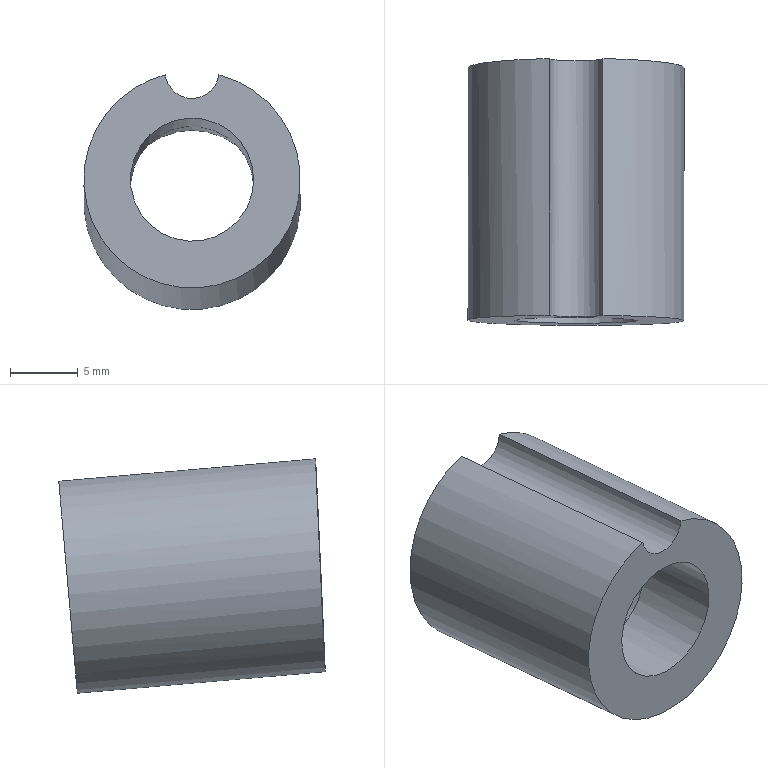Part | NX | features EKSD 16-20-9.100 2 | 1 solid | 7 faces | box 16 x 19.691 x 17.35 mm | volume 2155 mm3 | cylinder 4 | plane 3 | commonest cylinder face diameters 4 x1 9.1 x1 10.6 x1 16 x1
STEP:
#1=CARTESIAN_POINT('',(196.742,-27.508,-41.113));
#2=VERTEX_POINT('',#1);
#3=CARTESIAN_POINT('',(200.711,-27.508,-41.113));
#4=VERTEX_POINT('',#3);
#5=CARTESIAN_POINT('',(198.727,-27.486,-40.864));
#6=DIRECTION('',(0.,-0.9962,0.08716));
#7=DIRECTION('',(0.,-0.08716,-0.9962));
#8=AXIS2_PLACEMENT_3D('',#5,#6,#7);
#9=CIRCLE('',#8,2.);
#10=EDGE_CURVE('',#2,#4,#9,.T.);
#11=ORIENTED_EDGE('',*,*,#10,.T.);
#12=CARTESIAN_POINT('',(198.727,-28.184,-48.834));
#13=DIRECTION('',(0.,-0.9962,0.08716));
#14=DIRECTION('',(0.,-0.08716,-0.9962));
#15=AXIS2_PLACEMENT_3D('',#12,#13,#14);
#16=CIRCLE('',#15,8.);
#17=EDGE_CURVE('',#2,#4,#16,.T.);
#18=ORIENTED_EDGE('',*,*,#17,.F.);
#19=EDGE_LOOP('',(#11,#18));
#20=FACE_BOUND('',#19,.T.);
#21=CARTESIAN_POINT('',(198.727,-27.722,-43.554));
#22=VERTEX_POINT('',#21);
#23=CARTESIAN_POINT('',(198.727,-28.184,-48.834));
#24=DIRECTION('',(0.,0.9962,-0.08716));
#25=DIRECTION('',(0.,0.08716,0.9962));
#26=AXIS2_PLACEMENT_3D('',#23,#24,#25);
#27=CIRCLE('',#26,5.3);
#28=EDGE_CURVE('',#22,#22,#27,.T.);
#29=ORIENTED_EDGE('',*,*,#28,.F.);
#30=EDGE_LOOP('',(#29));
#31=FACE_BOUND('',#30,.T.);
#32=CARTESIAN_POINT('',(198.727,-28.184,-48.834));
#33=DIRECTION('',(0.,0.9962,-0.08716));
#34=DIRECTION('',(0.,0.08716,0.9962));
#35=AXIS2_PLACEMENT_3D('',#32,#33,#34);
#36=PLANE('',#35);
#37=ADVANCED_FACE('',(#20,#31),#36,.T.);
#38=CARTESIAN_POINT('',(200.711,-46.486,-39.453));
#39=VERTEX_POINT('',#38);
#40=CARTESIAN_POINT('',(196.742,-46.478,-39.454));
#41=VERTEX_POINT('',#40);
#42=CARTESIAN_POINT('',(198.727,-46.471,-39.203));
#43=DIRECTION('',(0.001957,0.999,-0.04546));
#44=DIRECTION('',(-0.04675,-0.04532,-0.9979));
#45=AXIS2_PLACEMENT_3D('',#42,#43,#44);
#46=ELLIPSE('',#45,2.002,2.);
#47=EDGE_CURVE('',#39,#41,#46,.T.);
#48=ORIENTED_EDGE('',*,*,#47,.T.);
#49=CARTESIAN_POINT('',(198.727,-46.835,-47.202));
#50=DIRECTION('',(0.001957,0.999,-0.04546));
#51=DIRECTION('',(-0.04675,-0.04532,-0.9979));
#52=AXIS2_PLACEMENT_3D('',#49,#50,#51);
#53=ELLIPSE('',#52,8.007,8.);
#54=EDGE_CURVE('',#39,#41,#53,.T.);
#55=ORIENTED_EDGE('',*,*,#54,.F.);
#56=EDGE_LOOP('',(#48,#55));
#57=FACE_BOUND('',#56,.T.);
#58=CARTESIAN_POINT('',(198.514,-47.041,-51.746));
#59=VERTEX_POINT('',#58);
#60=CARTESIAN_POINT('',(198.727,-46.835,-47.202));
#61=DIRECTION('',(0.001957,0.999,-0.04546));
#62=DIRECTION('',(-0.04675,-0.04532,-0.9979));
#63=AXIS2_PLACEMENT_3D('',#60,#61,#62);
#64=ELLIPSE('',#63,4.554,4.55);
#65=EDGE_CURVE('',#59,#59,#64,.F.);
#66=ORIENTED_EDGE('',*,*,#65,.F.);
#67=EDGE_LOOP('',(#66));
#68=FACE_BOUND('',#67,.T.);
#69=CARTESIAN_POINT('',(128.811,-48.589,-88.763));
#70=DIRECTION('',(0.001957,0.999,-0.04546));
#71=DIRECTION('',(0.06617,0.04523,0.9968));
#72=AXIS2_PLACEMENT_3D('',#69,#70,#71);
#73=PLANE('',#72);
#74=ADVANCED_FACE('',(#57,#68),#73,.F.);
#75=CARTESIAN_POINT('',(200.711,-37.47,-40.242));
#76=DIRECTION('',(0.,0.9962,-0.08716));
#77=VECTOR('',#76,1000.);
#78=LINE('',#75,#77);
#79=EDGE_CURVE('',#39,#4,#78,.T.);
#80=ORIENTED_EDGE('',*,*,#79,.F.);
#81=ORIENTED_EDGE('',*,*,#54,.T.);
#82=CARTESIAN_POINT('',(196.742,-37.47,-40.242));
#83=DIRECTION('',(0.,0.9962,-0.08716));
#84=VECTOR('',#83,1000.);
#85=LINE('',#82,#84);
#86=EDGE_CURVE('',#2,#41,#85,.F.);
#87=ORIENTED_EDGE('',*,*,#86,.F.);
#88=ORIENTED_EDGE('',*,*,#17,.T.);
#89=EDGE_LOOP('',(#80,#81,#87,#88));
#90=FACE_BOUND('',#89,.T.);
#91=CARTESIAN_POINT('',(198.727,-48.107,-47.091));
#92=DIRECTION('',(0.,0.9962,-0.08716));
#93=DIRECTION('',(0.,0.08716,0.9962));
#94=AXIS2_PLACEMENT_3D('',#91,#92,#93);
#95=CYLINDRICAL_SURFACE('',#94,8.);
#96=ADVANCED_FACE('',(#90),#95,.T.);
#97=CARTESIAN_POINT('',(198.727,-40.534,-52.321));
#98=VERTEX_POINT('',#97);
#99=CARTESIAN_POINT('',(198.727,-40.138,-47.788));
#100=DIRECTION('',(0.,-0.9962,0.08716));
#101=DIRECTION('',(0.,-0.08716,-0.9962));
#102=AXIS2_PLACEMENT_3D('',#99,#100,#101);
#103=CIRCLE('',#102,4.55);
#104=EDGE_CURVE('',#98,#98,#103,.F.);
#105=ORIENTED_EDGE('',*,*,#104,.T.);
#106=EDGE_LOOP('',(#105));
#107=FACE_BOUND('',#106,.T.);
#108=ORIENTED_EDGE('',*,*,#65,.T.);
#109=EDGE_LOOP('',(#108));
#110=FACE_BOUND('',#109,.T.);
#111=CARTESIAN_POINT('',(198.727,-49.104,-47.003));
#112=DIRECTION('',(0.,0.9962,-0.08716));
#113=DIRECTION('',(0.,0.08716,0.9962));
#114=AXIS2_PLACEMENT_3D('',#111,#112,#113);
#115=CYLINDRICAL_SURFACE('',#114,4.55);
#116=ADVANCED_FACE('',(#107,#110),#115,.F.);
#117=CARTESIAN_POINT('',(198.727,-39.676,-42.508));
#118=VERTEX_POINT('',#117);
#119=CARTESIAN_POINT('',(198.727,-40.138,-47.788));
#120=DIRECTION('',(0.,0.9962,-0.08716));
#121=DIRECTION('',(0.,0.08716,0.9962));
#122=AXIS2_PLACEMENT_3D('',#119,#120,#121);
#123=CIRCLE('',#122,5.3);
#124=EDGE_CURVE('',#118,#118,#123,.T.);
#125=ORIENTED_EDGE('',*,*,#124,.T.);
#126=EDGE_LOOP('',(#125));
#127=FACE_BOUND('',#126,.T.);
#128=ORIENTED_EDGE('',*,*,#104,.F.);
#129=EDGE_LOOP('',(#128));
#130=FACE_BOUND('',#129,.T.);
#131=CARTESIAN_POINT('',(198.727,-40.138,-47.788));
#132=DIRECTION('',(0.,-0.9962,0.08716));
#133=DIRECTION('',(0.,-0.08716,-0.9962));
#134=AXIS2_PLACEMENT_3D('',#131,#132,#133);
#135=PLANE('',#134);
#136=ADVANCED_FACE('',(#127,#130),#135,.F.);
#137=ORIENTED_EDGE('',*,*,#28,.T.);
#138=EDGE_LOOP('',(#137));
#139=FACE_BOUND('',#138,.T.);
#140=ORIENTED_EDGE('',*,*,#124,.F.);
#141=EDGE_LOOP('',(#140));
#142=FACE_BOUND('',#141,.T.);
#143=CARTESIAN_POINT('',(198.727,-40.138,-47.788));
#144=DIRECTION('',(0.,0.9962,-0.08716));
#145=DIRECTION('',(0.,0.08716,0.9962));
#146=AXIS2_PLACEMENT_3D('',#143,#144,#145);
#147=CYLINDRICAL_SURFACE('',#146,5.3);
#148=ADVANCED_FACE('',(#139,#142),#147,.F.);
#149=ORIENTED_EDGE('',*,*,#79,.T.);
#150=ORIENTED_EDGE('',*,*,#10,.F.);
#151=ORIENTED_EDGE('',*,*,#86,.T.);
#152=ORIENTED_EDGE('',*,*,#47,.F.);
#153=EDGE_LOOP('',(#149,#150,#151,#152));
#154=FACE_BOUND('',#153,.T.);
#155=CARTESIAN_POINT('',(198.727,-47.41,-39.121));
#156=DIRECTION('',(0.,0.9962,-0.08716));
#157=DIRECTION('',(0.,0.08716,0.9962));
#158=AXIS2_PLACEMENT_3D('',#155,#156,#157);
#159=CYLINDRICAL_SURFACE('',#158,2.);
#160=ADVANCED_FACE('',(#154),#159,.F.);
#161=CLOSED_SHELL('',(#37,#74,#96,#116,#136,#148,#160));
#162=MANIFOLD_SOLID_BREP('',#161);
#163=(LENGTH_UNIT()NAMED_UNIT(*)SI_UNIT(.MILLI.,.METRE.));
#164=UNCERTAINTY_MEASURE_WITH_UNIT(LENGTH_MEASURE(0.00001),#163,'','');
#165=(NAMED_UNIT(*)PLANE_ANGLE_UNIT()SI_UNIT($,.RADIAN.));
#166=(NAMED_UNIT(*)SI_UNIT($,.STERADIAN.)SOLID_ANGLE_UNIT());
#167=(GEOMETRIC_REPRESENTATION_CONTEXT(3)GLOBAL_UNCERTAINTY_ASSIGNED_CONTEXT((#164))GLOBAL_UNIT_ASSIGNED_CONTEXT((#163,#165,#166))REPRESENTATION_CONTEXT('',''));
#168=ADVANCED_BREP_SHAPE_REPRESENTATION('',(#162),#167);